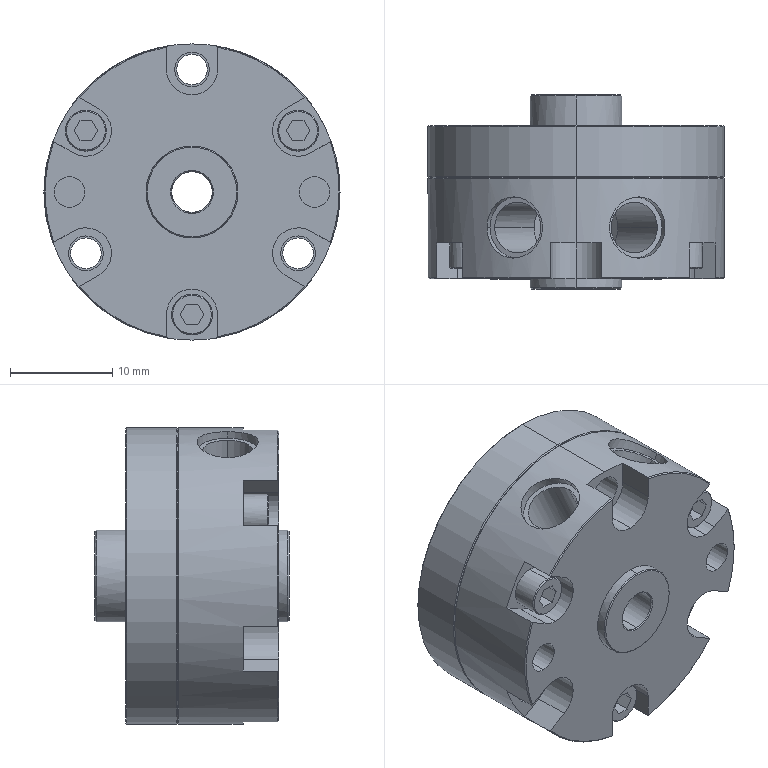Part | NX | 1 solid | 137 faces | box 29 x 19 x 29 mm | volume 8473 mm3 | cylinder 55 | plane 55 | cone 27 | commonest cylinder face diameters 5 x13 3 x10 4 x10 3.4 x6 6 x4 9 x4